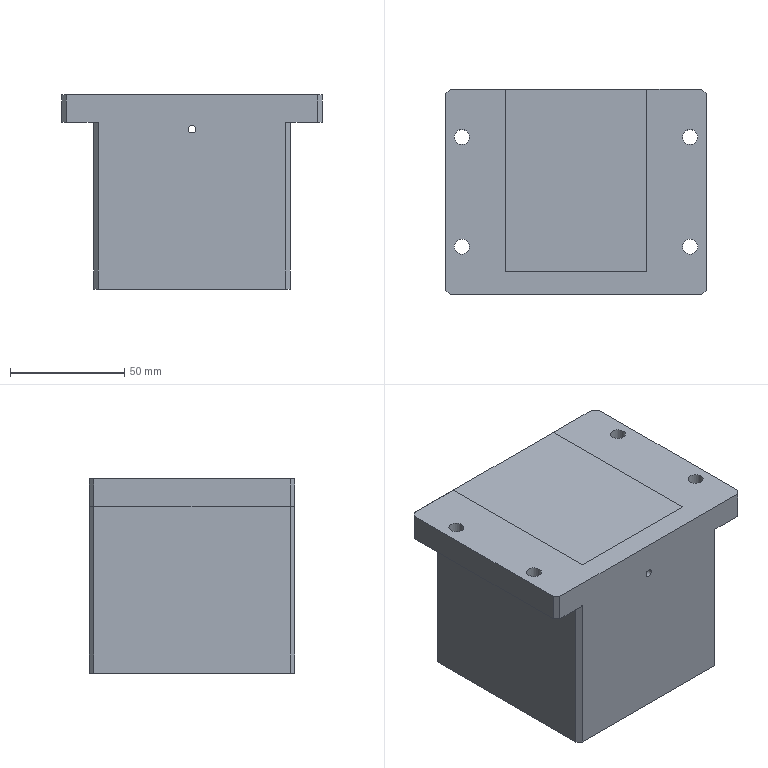CAM job | NX | 3+2 milling, drilling | part box 114 x 90 x 85 mm | stock box 119 x 100 x 90 mm
Tools:
number,name,description,diameter,corner_radius,flute_length,length,flutes
9,D10,平底铣刀-粗,10.0,0.0,35.0,75.0,2
17,D16,平底铣刀-粗,16.0,0.0,50.0,75.0,2
10,D10-J,平底铣刀-精,10.0,0.0,35.0,75.0,2
18,D16-J,平底铣刀-精,16.0,0.0,50.0,75.0,2
1,D80R0.8飞刀,圆鼻刀-粗,80.0,0.8,50.0,75.0,2
1,D80R0.8飞刀-J,圆鼻刀-精,80.0,0.8,50.0,75.0,2
2,D6倒角刀,倒角刀,6.0,0.0,3.0,25.0,2
19,M6X1.0,丝锥,5.0,0.0,35.0,50.0,2
15,ZT5,钻头,5.0,0.0,35.0,50.0,2
17,ZT6.6,钻头,6.6,0.0,35.0,50.0,2
3,D10-EXTENDED-J,平底铣刀-粗,10.0,0.0,50.0,75.0,2
Operations:
program,operation,operation_type,tool,method,geometry_group,spindle_rpm,surface_speed,feed_per_tooth,feed_cut,feed_plunge,cut_length_mm,path_length_mm,cut_time_min,machine_time_min
C,底壁铣分层开粗-中_COPY,VolumeBased25DMillingOperation,D16,分层开粗-切深K-步距G,W-C,5000.0,251.327,0.4,4000.0,100.0,48674.799,51430.627,12.169,12.444
C,等高光顺清角D6参考12_COPY,ZLevelMilling,D10-EXTENDED-J,分层精光-切深K-步距G,W-C,3000.0,94.248,0.2,1200.0,100.0,4738.226,5043.327,3.949,3.979
C,C0.3封闭铣廓倒角6X45L_COPY,PlanarMilling,D6倒角刀,爬面_倒角-切深0-步距G,W-C,7000.0,131.0,0.1071,1500.0,100.0,214.242,310.242,0.1428,0.1524
C,底壁铣精光底面-中_COPY,VolumeBased25DMillingOperation,D16-J,精光步距切深关,W-C,5000.0,251.327,0.1,1000.0,100.0,473.904,651.704,0.4739,0.4917
C,底壁铣精光侧面-中-选底面_COPY_2,VolumeBased25DMillingOperation,D16-J,侧刃精光-切深K-步距G,W-C,5000.0,251.327,0.1,1000.0,100.0,1635.61,2026.811,1.636,1.675
B,底壁铣飞面开粗_COPY,VolumeBased25DMillingOperation,D80R0.8飞刀,分层开粗-切深K-步距G,W-B,2800.0,703.696,0.5357,3000.0,100.0,4002.277,4312.86,1.334,1.365
B,底壁铣飞面精光_COPY,VolumeBased25DMillingOperation,D80R0.8飞刀-J,侧刃精光-切深K-步距G,W-B,4000.0,1005.28,0.125,1000.0,100.0,444.11,480.11,0.4441,0.4477
B,等高往复层切开粗-中_COPY,ZLevelMilling,D16,分层开粗-切深K-步距G,W-B,5000.0,251.327,0.4,4000.0,100.0,32359.751,32802.068,8.09,8.134
B,型腔铣开粗-中_COPY,CavityMilling,D10,分层开粗-切深K-步距G,W-B,8000.0,251.327,0.1875,3000.0,100.0,11512.326,11975.048,3.837,3.906
B,打点-深0.8_2,Operation,D6倒角刀,NONE,W-B,8000.0,150.796,0.0312,500.0,90.0,7.2,265.922,0.0144,0.0403
B,盲锥孔-M6螺纹底孔,Operation,ZT5,NONE,W-B,2500.0,39.27,0.03,150.0,90.0,70.009,391.539,0.4667,0.4989
B,铣倒角_2,PlanarMilling,D6倒角刀,METHOD,W-B,8000.0,150.796,0.0375,600.0,100.0,75.821,450.743,0.1264,0.1639
B,平面去毛刺6X45L_COPY,SurfaceContour,D6倒角刀,爬面_倒角-切深0-步距G,W-B,6500.0,122.519,0.1154,1500.0,100.0,580.624,1034.879,0.3871,0.4325
B,底壁铣倒角_COPY,VolumeBased25DMillingOperation,D6倒角刀,爬面_倒角-切深0-步距G,W-B,6500.0,122.519,0.1154,1500.0,100.0,238.432,277.832,0.159,0.1629
B,盲锥孔-攻牙M6,Operation,M6X1.0,METHOD,W-B,500.0,7.854,0.001,1.0,90.0,56.0,363.522,56.0,56.031
B,底壁铣精光侧面-中_COPY,VolumeBased25DMillingOperation,D10-J,侧刃精光-切深K-步距G,W-B,8000.0,251.32,0.0625,1000.0,100.0,149.991,201.452,0.15,0.1551
B,平面铣精光侧面-中_COPY_1,PlanarMilling,D10-J,侧刃精光-切深K-步距G,W-B,8000.0,251.32,0.0625,1000.0,100.0,175.851,220.851,0.1759,0.1804
B,底壁铣精光侧面-中-选底面_COPY,VolumeBased25DMillingOperation,D10-J,侧刃精光-切深K-步距G,W-B,8000.0,251.32,0.0625,1000.0,100.0,225.45,259.45,0.2255,0.2289
B,底壁铣精光侧面-中-选底面_COPY_1,VolumeBased25DMillingOperation,D16-J,侧刃精光-切深K-步距G,W-B,4000.0,201.062,0.125,1000.0,100.0,1933.889,5322.994,1.934,2.273
A,顶面,FaceMilling,D80R0.8飞刀,侧刃精光-切深K-步距G,W-A,4000.0,1005.31,0.125,1000.0,100.0,681.0,717.0,0.681,0.6846
A,外形粗_2,VolumeBased25DMillingOperation,D16,METHOD,W-A,5000.0,251.327,0.5,5000.0,80.0,49510.194,49633.993,9.902,9.914
A,打点-深0.8,Operation,D6倒角刀,NONE,W-A,8000.0,150.796,0.0312,500.0,90.0,7.2,253.426,0.0144,0.039
A,通孔-6-8,Operation,ZT6.6,NONE,W-A,2500.0,51.836,0.03,150.0,90.0,67.931,374.889,0.4529,0.4836
A,仅选体,SurfaceContour,D6倒角刀,METHOD,W-A,8000.0,150.796,0.1875,3000.0,100.0,420.615,456.416,0.1402,0.1438
A,铣倒角_1,PlanarMilling,D6倒角刀,METHOD,W-A,8000.0,150.796,0.05,800.0,100.0,92.54,452.586,0.1157,0.1517
A,外形半精_2,VolumeBased25DMillingOperation,D16-J,METHOD,W-A,5000.0,251.327,0.1,1000.0,100.0,2292.826,3009.667,2.293,2.365